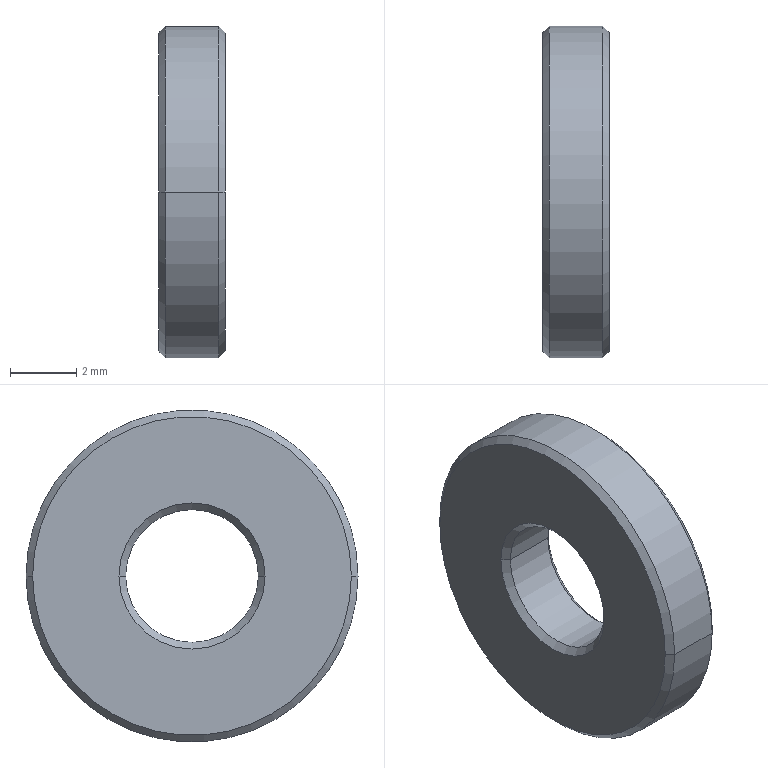Part | STEP file | wasmh10_4_2_2_03 | 1 solid | 14 faces | box 2 x 10 x 10 mm | volume 130.188 mm3 | cone 8 | cylinder 4 | plane 2 | commonest cylinder face diameters 4 x2 10 x2
STEP:
#1=CARTESIAN_POINT('',(0.,0.,0.));
#2=DIRECTION('',(0.,0.,1.));
#3=DIRECTION('',(1.,0.,0.));
#4=AXIS2_PLACEMENT_3D('',#1,#2,#3);
#5=CARTESIAN_POINT('',(2.,4.8,0.));
#6=VERTEX_POINT('',#5);
#7=CARTESIAN_POINT('',(2.,-4.8,0.));
#8=VERTEX_POINT('',#7);
#9=CARTESIAN_POINT('',(2.,0.,0.));
#10=DIRECTION('',(1.,0.,0.));
#11=DIRECTION('',(0.,-1.,0.));
#12=AXIS2_PLACEMENT_3D('',#9,#10,#11);
#13=CIRCLE('',#12,4.8);
#14=CARTESIAN_POINT('',(1.8,0.,0.));
#15=DIRECTION('',(-1.,0.,0.));
#16=DIRECTION('',(0.,-1.,0.));
#17=AXIS2_PLACEMENT_3D('',#14,#15,#16);
#18=CONICAL_SURFACE('',#17,5.,0.7854);
#19=CARTESIAN_POINT('',(6.283,-0.2));
#20=DIRECTION('',(-1.,0.));
#21=VECTOR('',#20,1.);
#22=LINE('',#19,#21);
#23=(GEOMETRIC_REPRESENTATION_CONTEXT(2)PARAMETRIC_REPRESENTATION_CONTEXT()REPRESENTATION_CONTEXT('',''));
#24=DEFINITIONAL_REPRESENTATION('',(#22),#23);
#25=PCURVE('',#18,#24);
#26=CARTESIAN_POINT('',(2.,-3.5,0.));
#27=DIRECTION('',(1.,0.,0.));
#28=DIRECTION('',(0.,1.,0.));
#29=AXIS2_PLACEMENT_3D('',#26,#27,#28);
#30=PLANE('',#29);
#31=CARTESIAN_POINT('',(3.5,0.));
#32=DIRECTION('',(-1.,0.));
#33=AXIS2_PLACEMENT_2D('',#31,#32);
#34=CIRCLE('',#33,4.8);
#35=(GEOMETRIC_REPRESENTATION_CONTEXT(2)PARAMETRIC_REPRESENTATION_CONTEXT()REPRESENTATION_CONTEXT('',''));
#36=DEFINITIONAL_REPRESENTATION('',(#34),#35);
#37=PCURVE('',#30,#36);
#38=SURFACE_CURVE('',#13,(#25,#37),.PCURVE_S1.);
#39=EDGE_CURVE('',#6,#8,#38,.T.);
#40=ORIENTED_EDGE('',*,*,#39,.F.);
#41=CARTESIAN_POINT('',(1.8,5.,0.));
#42=VERTEX_POINT('',#41);
#43=CARTESIAN_POINT('',(1.8,5.,0.));
#44=DIRECTION('',(-0.7071,0.7071,0.));
#45=VECTOR('',#44,1.);
#46=LINE('',#43,#45);
#47=CARTESIAN_POINT('',(3.142,0.));
#48=DIRECTION('',(0.,1.));
#49=VECTOR('',#48,1.);
#50=LINE('',#47,#49);
#51=(GEOMETRIC_REPRESENTATION_CONTEXT(2)PARAMETRIC_REPRESENTATION_CONTEXT()REPRESENTATION_CONTEXT('',''));
#52=DEFINITIONAL_REPRESENTATION('',(#50),#51);
#53=PCURVE('',#18,#52);
#54=CARTESIAN_POINT('',(1.8,0.,0.));
#55=DIRECTION('',(-1.,0.,0.));
#56=DIRECTION('',(0.,-1.,0.));
#57=AXIS2_PLACEMENT_3D('',#54,#55,#56);
#58=CONICAL_SURFACE('',#57,5.,0.7854);
#59=CARTESIAN_POINT('',(3.142,0.));
#60=DIRECTION('',(0.,1.));
#61=VECTOR('',#60,1.);
#62=LINE('',#59,#61);
#63=(GEOMETRIC_REPRESENTATION_CONTEXT(2)PARAMETRIC_REPRESENTATION_CONTEXT()REPRESENTATION_CONTEXT('',''));
#64=DEFINITIONAL_REPRESENTATION('',(#62),#63);
#65=PCURVE('',#58,#64);
#66=SURFACE_CURVE('',#46,(#53,#65),.PCURVE_S1.);
#67=EDGE_CURVE('',#6,#42,#66,.T.);
#68=ORIENTED_EDGE('',*,*,#67,.T.);
#69=CARTESIAN_POINT('',(1.8,-5.,0.));
#70=VERTEX_POINT('',#69);
#71=CARTESIAN_POINT('',(1.8,0.,0.));
#72=DIRECTION('',(1.,0.,0.));
#73=DIRECTION('',(0.,-1.,0.));
#74=AXIS2_PLACEMENT_3D('',#71,#72,#73);
#75=CIRCLE('',#74,5.);
#76=CARTESIAN_POINT('',(6.283,0.));
#77=DIRECTION('',(-1.,0.));
#78=VECTOR('',#77,1.);
#79=LINE('',#76,#78);
#80=(GEOMETRIC_REPRESENTATION_CONTEXT(2)PARAMETRIC_REPRESENTATION_CONTEXT()REPRESENTATION_CONTEXT('',''));
#81=DEFINITIONAL_REPRESENTATION('',(#79),#80);
#82=PCURVE('',#18,#81);
#83=CARTESIAN_POINT('',(1.,0.,0.));
#84=DIRECTION('',(-1.,0.,0.));
#85=DIRECTION('',(0.,-1.,0.));
#86=AXIS2_PLACEMENT_3D('',#83,#84,#85);
#87=CYLINDRICAL_SURFACE('',#86,5.);
#88=CARTESIAN_POINT('',(6.283,-0.8));
#89=DIRECTION('',(-1.,0.));
#90=VECTOR('',#89,1.);
#91=LINE('',#88,#90);
#92=(GEOMETRIC_REPRESENTATION_CONTEXT(2)PARAMETRIC_REPRESENTATION_CONTEXT()REPRESENTATION_CONTEXT('',''));
#93=DEFINITIONAL_REPRESENTATION('',(#91),#92);
#94=PCURVE('',#87,#93);
#95=SURFACE_CURVE('',#75,(#82,#94),.PCURVE_S1.);
#96=EDGE_CURVE('',#42,#70,#95,.T.);
#97=ORIENTED_EDGE('',*,*,#96,.T.);
#98=CARTESIAN_POINT('',(1.8,-5.,0.));
#99=DIRECTION('',(-0.7071,-0.7071,0.));
#100=VECTOR('',#99,1.);
#101=LINE('',#98,#100);
#102=CARTESIAN_POINT('',(0.,0.));
#103=DIRECTION('',(0.,1.));
#104=VECTOR('',#103,1.);
#105=LINE('',#102,#104);
#106=(GEOMETRIC_REPRESENTATION_CONTEXT(2)PARAMETRIC_REPRESENTATION_CONTEXT()REPRESENTATION_CONTEXT('',''));
#107=DEFINITIONAL_REPRESENTATION('',(#105),#106);
#108=PCURVE('',#18,#107);
#109=CARTESIAN_POINT('',(6.283,0.));
#110=DIRECTION('',(0.,1.));
#111=VECTOR('',#110,1.);
#112=LINE('',#109,#111);
#113=(GEOMETRIC_REPRESENTATION_CONTEXT(2)PARAMETRIC_REPRESENTATION_CONTEXT()REPRESENTATION_CONTEXT('',''));
#114=DEFINITIONAL_REPRESENTATION('',(#112),#113);
#115=PCURVE('',#58,#114);
#116=SURFACE_CURVE('',#101,(#108,#115),.PCURVE_S1.);
#117=EDGE_CURVE('',#8,#70,#116,.T.);
#118=ORIENTED_EDGE('',*,*,#117,.F.);
#119=EDGE_LOOP('',(#40,#68,#97,#118));
#120=FACE_BOUND('',#119,.T.);
#121=ADVANCED_FACE('',(#120),#18,.T.);
#122=CARTESIAN_POINT('',(1.8,2.,0.));
#123=VERTEX_POINT('',#122);
#124=CARTESIAN_POINT('',(2.,2.2,0.));
#125=VERTEX_POINT('',#124);
#126=CARTESIAN_POINT('',(2.,2.2,0.));
#127=DIRECTION('',(0.7071,0.7071,0.));
#128=VECTOR('',#127,1.);
#129=LINE('',#126,#128);
#130=CARTESIAN_POINT('',(2.,0.,0.));
#131=DIRECTION('',(1.,0.,0.));
#132=DIRECTION('',(0.,1.,0.));
#133=AXIS2_PLACEMENT_3D('',#130,#131,#132);
#134=CONICAL_SURFACE('',#133,2.2,0.7854);
#135=CARTESIAN_POINT('',(6.283,0.));
#136=DIRECTION('',(0.,1.));
#137=VECTOR('',#136,1.);
#138=LINE('',#135,#137);
#139=(GEOMETRIC_REPRESENTATION_CONTEXT(2)PARAMETRIC_REPRESENTATION_CONTEXT()REPRESENTATION_CONTEXT('',''));
#140=DEFINITIONAL_REPRESENTATION('',(#138),#139);
#141=PCURVE('',#134,#140);
#142=CARTESIAN_POINT('',(2.,0.,0.));
#143=DIRECTION('',(1.,0.,0.));
#144=DIRECTION('',(0.,1.,0.));
#145=AXIS2_PLACEMENT_3D('',#142,#143,#144);
#146=CONICAL_SURFACE('',#145,2.2,0.7854);
#147=CARTESIAN_POINT('',(0.,0.));
#148=DIRECTION('',(0.,1.));
#149=VECTOR('',#148,1.);
#150=LINE('',#147,#149);
#151=(GEOMETRIC_REPRESENTATION_CONTEXT(2)PARAMETRIC_REPRESENTATION_CONTEXT()REPRESENTATION_CONTEXT('',''));
#152=DEFINITIONAL_REPRESENTATION('',(#150),#151);
#153=PCURVE('',#146,#152);
#154=SURFACE_CURVE('',#129,(#141,#153),.PCURVE_S1.);
#155=EDGE_CURVE('',#123,#125,#154,.T.);
#156=ORIENTED_EDGE('',*,*,#155,.T.);
#157=CARTESIAN_POINT('',(2.,-2.2,0.));
#158=VERTEX_POINT('',#157);
#159=CARTESIAN_POINT('',(2.,0.,0.));
#160=DIRECTION('',(-1.,0.,0.));
#161=DIRECTION('',(0.,1.,0.));
#162=AXIS2_PLACEMENT_3D('',#159,#160,#161);
#163=CIRCLE('',#162,2.2);
#164=CARTESIAN_POINT('',(6.283,0.));
#165=DIRECTION('',(-1.,0.));
#166=VECTOR('',#165,1.);
#167=LINE('',#164,#166);
#168=(GEOMETRIC_REPRESENTATION_CONTEXT(2)PARAMETRIC_REPRESENTATION_CONTEXT()REPRESENTATION_CONTEXT('',''));
#169=DEFINITIONAL_REPRESENTATION('',(#167),#168);
#170=PCURVE('',#134,#169);
#171=CARTESIAN_POINT('',(5.7,0.));
#172=CARTESIAN_POINT('',(5.7,-3.811));
#173=CARTESIAN_POINT('',(2.4,-1.905));
#174=CARTESIAN_POINT('',(-0.9,0.));
#175=CARTESIAN_POINT('',(2.4,1.905));
#176=CARTESIAN_POINT('',(5.7,3.811));
#177=CARTESIAN_POINT('',(5.7,0.));
#178=(BOUNDED_CURVE()B_SPLINE_CURVE(2,(#171,#172,#173,#174,#175,#176,#177),.UNSPECIFIED.,.T.,.F.)B_SPLINE_CURVE_WITH_KNOTS((1,2,2,2,2,1),(-2.094,0.,2.094,4.189,6.283,8.378),.UNSPECIFIED.)CURVE()GEOMETRIC_REPRESENTATION_ITEM()RATIONAL_B_SPLINE_CURVE((1.,0.5,1.,0.5,1.,0.5,1.))REPRESENTATION_ITEM(''));
#179=(GEOMETRIC_REPRESENTATION_CONTEXT(2)PARAMETRIC_REPRESENTATION_CONTEXT()REPRESENTATION_CONTEXT('',''));
#180=DEFINITIONAL_REPRESENTATION('',(#178),#179);
#181=PCURVE('',#30,#180);
#182=SURFACE_CURVE('',#163,(#170,#181),.PCURVE_S1.);
#183=EDGE_CURVE('',#125,#158,#182,.T.);
#184=ORIENTED_EDGE('',*,*,#183,.T.);
#185=CARTESIAN_POINT('',(1.8,-2.,0.));
#186=VERTEX_POINT('',#185);
#187=CARTESIAN_POINT('',(2.,-2.2,0.));
#188=DIRECTION('',(0.7071,-0.7071,0.));
#189=VECTOR('',#188,1.);
#190=LINE('',#187,#189);
#191=CARTESIAN_POINT('',(3.142,0.));
#192=DIRECTION('',(0.,1.));
#193=VECTOR('',#192,1.);
#194=LINE('',#191,#193);
#195=(GEOMETRIC_REPRESENTATION_CONTEXT(2)PARAMETRIC_REPRESENTATION_CONTEXT()REPRESENTATION_CONTEXT('',''));
#196=DEFINITIONAL_REPRESENTATION('',(#194),#195);
#197=PCURVE('',#134,#196);
#198=CARTESIAN_POINT('',(3.142,0.));
#199=DIRECTION('',(0.,1.));
#200=VECTOR('',#199,1.);
#201=LINE('',#198,#200);
#202=(GEOMETRIC_REPRESENTATION_CONTEXT(2)PARAMETRIC_REPRESENTATION_CONTEXT()REPRESENTATION_CONTEXT('',''));
#203=DEFINITIONAL_REPRESENTATION('',(#201),#202);
#204=PCURVE('',#146,#203);
#205=SURFACE_CURVE('',#190,(#197,#204),.PCURVE_S1.);
#206=EDGE_CURVE('',#186,#158,#205,.T.);
#207=ORIENTED_EDGE('',*,*,#206,.F.);
#208=CARTESIAN_POINT('',(1.8,0.,0.));
#209=DIRECTION('',(1.,0.,0.));
#210=DIRECTION('',(0.,-1.,0.));
#211=AXIS2_PLACEMENT_3D('',#208,#209,#210);
#212=CIRCLE('',#211,2.);
#213=CARTESIAN_POINT('',(3.142,-0.2));
#214=DIRECTION('',(1.,0.));
#215=VECTOR('',#214,1.);
#216=LINE('',#213,#215);
#217=(GEOMETRIC_REPRESENTATION_CONTEXT(2)PARAMETRIC_REPRESENTATION_CONTEXT()REPRESENTATION_CONTEXT('',''));
#218=DEFINITIONAL_REPRESENTATION('',(#216),#217);
#219=PCURVE('',#134,#218);
#220=CARTESIAN_POINT('',(1.,0.,0.));
#221=DIRECTION('',(-1.,0.,0.));
#222=DIRECTION('',(0.,-1.,0.));
#223=AXIS2_PLACEMENT_3D('',#220,#221,#222);
#224=CYLINDRICAL_SURFACE('',#223,2.);
#225=CARTESIAN_POINT('',(6.283,-0.8));
#226=DIRECTION('',(-1.,0.));
#227=VECTOR('',#226,1.);
#228=LINE('',#225,#227);
#229=(GEOMETRIC_REPRESENTATION_CONTEXT(2)PARAMETRIC_REPRESENTATION_CONTEXT()REPRESENTATION_CONTEXT('',''));
#230=DEFINITIONAL_REPRESENTATION('',(#228),#229);
#231=PCURVE('',#224,#230);
#232=SURFACE_CURVE('',#212,(#219,#231),.PCURVE_S1.);
#233=EDGE_CURVE('',#186,#123,#232,.T.);
#234=ORIENTED_EDGE('',*,*,#233,.T.);
#235=EDGE_LOOP('',(#156,#184,#207,#234));
#236=FACE_BOUND('',#235,.F.);
#237=ADVANCED_FACE('',(#236),#134,.F.);
#238=ORIENTED_EDGE('',*,*,#96,.F.);
#239=CARTESIAN_POINT('',(0.2,5.,0.));
#240=VERTEX_POINT('',#239);
#241=CARTESIAN_POINT('',(1.,5.,0.));
#242=DIRECTION('',(-1.,0.,0.));
#243=VECTOR('',#242,1.);
#244=LINE('',#241,#243);
#245=CARTESIAN_POINT('',(3.142,0.));
#246=DIRECTION('',(0.,1.));
#247=VECTOR('',#246,1.);
#248=LINE('',#245,#247);
#249=(GEOMETRIC_REPRESENTATION_CONTEXT(2)PARAMETRIC_REPRESENTATION_CONTEXT()REPRESENTATION_CONTEXT('',''));
#250=DEFINITIONAL_REPRESENTATION('',(#248),#249);
#251=PCURVE('',#87,#250);
#252=CARTESIAN_POINT('',(1.,0.,0.));
#253=DIRECTION('',(-1.,0.,0.));
#254=DIRECTION('',(0.,-1.,0.));
#255=AXIS2_PLACEMENT_3D('',#252,#253,#254);
#256=CYLINDRICAL_SURFACE('',#255,5.);
#257=CARTESIAN_POINT('',(3.142,0.));
#258=DIRECTION('',(0.,1.));
#259=VECTOR('',#258,1.);
#260=LINE('',#257,#259);
#261=(GEOMETRIC_REPRESENTATION_CONTEXT(2)PARAMETRIC_REPRESENTATION_CONTEXT()REPRESENTATION_CONTEXT('',''));
#262=DEFINITIONAL_REPRESENTATION('',(#260),#261);
#263=PCURVE('',#256,#262);
#264=SURFACE_CURVE('',#244,(#251,#263),.PCURVE_S1.);
#265=EDGE_CURVE('',#42,#240,#264,.T.);
#266=ORIENTED_EDGE('',*,*,#265,.T.);
#267=CARTESIAN_POINT('',(0.2,-5.,0.));
#268=VERTEX_POINT('',#267);
#269=CARTESIAN_POINT('',(0.2,0.,0.));
#270=DIRECTION('',(1.,0.,0.));
#271=DIRECTION('',(0.,-1.,0.));
#272=AXIS2_PLACEMENT_3D('',#269,#270,#271);
#273=CIRCLE('',#272,5.);
#274=CARTESIAN_POINT('',(6.283,0.8));
#275=DIRECTION('',(-1.,0.));
#276=VECTOR('',#275,1.);
#277=LINE('',#274,#276);
#278=(GEOMETRIC_REPRESENTATION_CONTEXT(2)PARAMETRIC_REPRESENTATION_CONTEXT()REPRESENTATION_CONTEXT('',''));
#279=DEFINITIONAL_REPRESENTATION('',(#277),#278);
#280=PCURVE('',#87,#279);
#281=CARTESIAN_POINT('',(0.2,0.,0.));
#282=DIRECTION('',(1.,0.,0.));
#283=DIRECTION('',(0.,1.,0.));
#284=AXIS2_PLACEMENT_3D('',#281,#282,#283);
#285=CONICAL_SURFACE('',#284,5.,0.7854);
#286=CARTESIAN_POINT('',(-3.142,0.));
#287=DIRECTION('',(1.,0.));
#288=VECTOR('',#287,1.);
#289=LINE('',#286,#288);
#290=(GEOMETRIC_REPRESENTATION_CONTEXT(2)PARAMETRIC_REPRESENTATION_CONTEXT()REPRESENTATION_CONTEXT('',''));
#291=DEFINITIONAL_REPRESENTATION('',(#289),#290);
#292=PCURVE('',#285,#291);
#293=SURFACE_CURVE('',#273,(#280,#292),.PCURVE_S1.);
#294=EDGE_CURVE('',#240,#268,#293,.T.);
#295=ORIENTED_EDGE('',*,*,#294,.T.);
#296=CARTESIAN_POINT('',(1.,-5.,0.));
#297=DIRECTION('',(-1.,0.,0.));
#298=VECTOR('',#297,1.);
#299=LINE('',#296,#298);
#300=CARTESIAN_POINT('',(0.,0.));
#301=DIRECTION('',(0.,1.));
#302=VECTOR('',#301,1.);
#303=LINE('',#300,#302);
#304=(GEOMETRIC_REPRESENTATION_CONTEXT(2)PARAMETRIC_REPRESENTATION_CONTEXT()REPRESENTATION_CONTEXT('',''));
#305=DEFINITIONAL_REPRESENTATION('',(#303),#304);
#306=PCURVE('',#87,#305);
#307=CARTESIAN_POINT('',(6.283,0.));
#308=DIRECTION('',(0.,1.));
#309=VECTOR('',#308,1.);
#310=LINE('',#307,#309);
#311=(GEOMETRIC_REPRESENTATION_CONTEXT(2)PARAMETRIC_REPRESENTATION_CONTEXT()REPRESENTATION_CONTEXT('',''));
#312=DEFINITIONAL_REPRESENTATION('',(#310),#311);
#313=PCURVE('',#256,#312);
#314=SURFACE_CURVE('',#299,(#306,#313),.PCURVE_S1.);
#315=EDGE_CURVE('',#70,#268,#314,.T.);
#316=ORIENTED_EDGE('',*,*,#315,.F.);
#317=EDGE_LOOP('',(#238,#266,#295,#316));
#318=FACE_BOUND('',#317,.T.);
#319=ADVANCED_FACE('',(#318),#87,.T.);
#320=CARTESIAN_POINT('',(0.2,-2.,0.));
#321=VERTEX_POINT('',#320);
#322=CARTESIAN_POINT('',(1.,-2.,0.));
#323=DIRECTION('',(-1.,0.,0.));
#324=VECTOR('',#323,1.);
#325=LINE('',#322,#324);
#326=CARTESIAN_POINT('',(6.283,0.));
#327=DIRECTION('',(0.,1.));
#328=VECTOR('',#327,1.);
#329=LINE('',#326,#328);
#330=(GEOMETRIC_REPRESENTATION_CONTEXT(2)PARAMETRIC_REPRESENTATION_CONTEXT()REPRESENTATION_CONTEXT('',''));
#331=DEFINITIONAL_REPRESENTATION('',(#329),#330);
#332=PCURVE('',#224,#331);
#333=CARTESIAN_POINT('',(1.,0.,0.));
#334=DIRECTION('',(-1.,0.,0.));
#335=DIRECTION('',(0.,-1.,0.));
#336=AXIS2_PLACEMENT_3D('',#333,#334,#335);
#337=CYLINDRICAL_SURFACE('',#336,2.);
#338=CARTESIAN_POINT('',(0.,0.));
#339=DIRECTION('',(0.,1.));
#340=VECTOR('',#339,1.);
#341=LINE('',#338,#340);
#342=(GEOMETRIC_REPRESENTATION_CONTEXT(2)PARAMETRIC_REPRESENTATION_CONTEXT()REPRESENTATION_CONTEXT('',''));
#343=DEFINITIONAL_REPRESENTATION('',(#341),#342);
#344=PCURVE('',#337,#343);
#345=SURFACE_CURVE('',#325,(#332,#344),.PCURVE_S1.);
#346=EDGE_CURVE('',#186,#321,#345,.T.);
#347=ORIENTED_EDGE('',*,*,#346,.T.);
#348=CARTESIAN_POINT('',(0.2,2.,0.));
#349=VERTEX_POINT('',#348);
#350=CARTESIAN_POINT('',(0.2,0.,0.));
#351=DIRECTION('',(1.,0.,0.));
#352=DIRECTION('',(0.,-1.,0.));
#353=AXIS2_PLACEMENT_3D('',#350,#351,#352);
#354=CIRCLE('',#353,2.);
#355=CARTESIAN_POINT('',(6.283,0.8));
#356=DIRECTION('',(-1.,0.));
#357=VECTOR('',#356,1.);
#358=LINE('',#355,#357);
#359=(GEOMETRIC_REPRESENTATION_CONTEXT(2)PARAMETRIC_REPRESENTATION_CONTEXT()REPRESENTATION_CONTEXT('',''));
#360=DEFINITIONAL_REPRESENTATION('',(#358),#359);
#361=PCURVE('',#224,#360);
#362=CARTESIAN_POINT('',(0.,0.,0.));
#363=DIRECTION('',(-1.,0.,0.));
#364=DIRECTION('',(0.,-1.,0.));
#365=AXIS2_PLACEMENT_3D('',#362,#363,#364);
#366=CONICAL_SURFACE('',#365,2.2,0.7854);
#367=CARTESIAN_POINT('',(6.283,-0.2));
#368=DIRECTION('',(-1.,0.));
#369=VECTOR('',#368,1.);
#370=LINE('',#367,#369);
#371=(GEOMETRIC_REPRESENTATION_CONTEXT(2)PARAMETRIC_REPRESENTATION_CONTEXT()REPRESENTATION_CONTEXT('',''));
#372=DEFINITIONAL_REPRESENTATION('',(#370),#371);
#373=PCURVE('',#366,#372);
#374=SURFACE_CURVE('',#354,(#361,#373),.PCURVE_S1.);
#375=EDGE_CURVE('',#321,#349,#374,.T.);
#376=ORIENTED_EDGE('',*,*,#375,.T.);
#377=CARTESIAN_POINT('',(1.,2.,0.));
#378=DIRECTION('',(-1.,0.,0.));
#379=VECTOR('',#378,1.);
#380=LINE('',#377,#379);
#381=CARTESIAN_POINT('',(3.142,0.));
#382=DIRECTION('',(0.,1.));
#383=VECTOR('',#382,1.);
#384=LINE('',#381,#383);
#385=(GEOMETRIC_REPRESENTATION_CONTEXT(2)PARAMETRIC_REPRESENTATION_CONTEXT()REPRESENTATION_CONTEXT('',''));
#386=DEFINITIONAL_REPRESENTATION('',(#384),#385);
#387=PCURVE('',#224,#386);
#388=CARTESIAN_POINT('',(3.142,0.));
#389=DIRECTION('',(0.,1.));
#390=VECTOR('',#389,1.);
#391=LINE('',#388,#390);
#392=(GEOMETRIC_REPRESENTATION_CONTEXT(2)PARAMETRIC_REPRESENTATION_CONTEXT()REPRESENTATION_CONTEXT('',''));
#393=DEFINITIONAL_REPRESENTATION('',(#391),#392);
#394=PCURVE('',#337,#393);
#395=SURFACE_CURVE('',#380,(#387,#394),.PCURVE_S1.);
#396=EDGE_CURVE('',#123,#349,#395,.T.);
#397=ORIENTED_EDGE('',*,*,#396,.F.);
#398=ORIENTED_EDGE('',*,*,#233,.F.);
#399=EDGE_LOOP('',(#347,#376,#397,#398));
#400=FACE_BOUND('',#399,.F.);
#401=ADVANCED_FACE('',(#400),#224,.F.);
#402=CARTESIAN_POINT('',(0.,4.8,0.));
#403=VERTEX_POINT('',#402);
#404=CARTESIAN_POINT('',(0.,-4.8,0.));
#405=VERTEX_POINT('',#404);
#406=CARTESIAN_POINT('',(0.,0.,0.));
#407=DIRECTION('',(1.,0.,0.));
#408=DIRECTION('',(0.,1.,0.));
#409=AXIS2_PLACEMENT_3D('',#406,#407,#408);
#410=CIRCLE('',#409,4.8);
#411=CARTESIAN_POINT('',(0.,-0.2));
#412=DIRECTION('',(1.,0.));
#413=VECTOR('',#412,1.);
#414=LINE('',#411,#413);
#415=(GEOMETRIC_REPRESENTATION_CONTEXT(2)PARAMETRIC_REPRESENTATION_CONTEXT()REPRESENTATION_CONTEXT('',''));
#416=DEFINITIONAL_REPRESENTATION('',(#414),#415);
#417=PCURVE('',#285,#416);
#418=CARTESIAN_POINT('',(0.,-3.5,0.));
#419=DIRECTION('',(-1.,0.,0.));
#420=DIRECTION('',(0.,-1.,0.));
#421=AXIS2_PLACEMENT_3D('',#418,#419,#420);
#422=PLANE('',#421);
#423=CARTESIAN_POINT('',(-8.3,0.));
#424=CARTESIAN_POINT('',(-8.3,8.314));
#425=CARTESIAN_POINT('',(-1.1,4.157));
#426=CARTESIAN_POINT('',(6.1,0.));
#427=CARTESIAN_POINT('',(-1.1,-4.157));
#428=CARTESIAN_POINT('',(-8.3,-8.314));
#429=CARTESIAN_POINT('',(-8.3,0.));
#430=(BOUNDED_CURVE()B_SPLINE_CURVE(2,(#423,#424,#425,#426,#427,#428,#429),.UNSPECIFIED.,.T.,.F.)B_SPLINE_CURVE_WITH_KNOTS((1,2,2,2,2,1),(-2.094,0.,2.094,4.189,6.283,8.378),.UNSPECIFIED.)CURVE()GEOMETRIC_REPRESENTATION_ITEM()RATIONAL_B_SPLINE_CURVE((1.,0.5,1.,0.5,1.,0.5,1.))REPRESENTATION_ITEM(''));
#431=(GEOMETRIC_REPRESENTATION_CONTEXT(2)PARAMETRIC_REPRESENTATION_CONTEXT()REPRESENTATION_CONTEXT('',''));
#432=DEFINITIONAL_REPRESENTATION('',(#430),#431);
#433=PCURVE('',#422,#432);
#434=SURFACE_CURVE('',#410,(#417,#433),.PCURVE_S1.);
#435=EDGE_CURVE('',#403,#405,#434,.T.);
#436=ORIENTED_EDGE('',*,*,#435,.T.);
#437=CARTESIAN_POINT('',(0.2,-5.,0.));
#438=DIRECTION('',(0.7071,-0.7071,0.));
#439=VECTOR('',#438,1.);
#440=LINE('',#437,#439);
#441=CARTESIAN_POINT('',(3.142,0.));
#442=DIRECTION('',(0.,1.));
#443=VECTOR('',#442,1.);
#444=LINE('',#441,#443);
#445=(GEOMETRIC_REPRESENTATION_CONTEXT(2)PARAMETRIC_REPRESENTATION_CONTEXT()REPRESENTATION_CONTEXT('',''));
#446=DEFINITIONAL_REPRESENTATION('',(#444),#445);
#447=PCURVE('',#285,#446);
#448=CARTESIAN_POINT('',(0.2,0.,0.));
#449=DIRECTION('',(1.,0.,0.));
#450=DIRECTION('',(0.,1.,0.));
#451=AXIS2_PLACEMENT_3D('',#448,#449,#450);
#452=CONICAL_SURFACE('',#451,5.,0.7854);
#453=CARTESIAN_POINT('',(3.142,0.));
#454=DIRECTION('',(0.,1.));
#455=VECTOR('',#454,1.);
#456=LINE('',#453,#455);
#457=(GEOMETRIC_REPRESENTATION_CONTEXT(2)PARAMETRIC_REPRESENTATION_CONTEXT()REPRESENTATION_CONTEXT('',''));
#458=DEFINITIONAL_REPRESENTATION('',(#456),#457);
#459=PCURVE('',#452,#458);
#460=SURFACE_CURVE('',#440,(#447,#459),.PCURVE_S1.);
#461=EDGE_CURVE('',#405,#268,#460,.T.);
#462=ORIENTED_EDGE('',*,*,#461,.T.);
#463=ORIENTED_EDGE('',*,*,#294,.F.);
#464=CARTESIAN_POINT('',(0.2,5.,0.));
#465=DIRECTION('',(0.7071,0.7071,0.));
#466=VECTOR('',#465,1.);
#467=LINE('',#464,#466);
#468=CARTESIAN_POINT('',(0.,0.));
#469=DIRECTION('',(0.,1.));
#470=VECTOR('',#469,1.);
#471=LINE('',#468,#470);
#472=(GEOMETRIC_REPRESENTATION_CONTEXT(2)PARAMETRIC_REPRESENTATION_CONTEXT()REPRESENTATION_CONTEXT('',''));
#473=DEFINITIONAL_REPRESENTATION('',(#471),#472);
#474=PCURVE('',#285,#473);
#475=CARTESIAN_POINT('',(6.283,0.));
#476=DIRECTION('',(0.,1.));
#477=VECTOR('',#476,1.);
#478=LINE('',#475,#477);
#479=(GEOMETRIC_REPRESENTATION_CONTEXT(2)PARAMETRIC_REPRESENTATION_CONTEXT()REPRESENTATION_CONTEXT('',''));
#480=DEFINITIONAL_REPRESENTATION('',(#478),#479);
#481=PCURVE('',#452,#480);
#482=SURFACE_CURVE('',#467,(#474,#481),.PCURVE_S1.);
#483=EDGE_CURVE('',#403,#240,#482,.T.);
#484=ORIENTED_EDGE('',*,*,#483,.F.);
#485=EDGE_LOOP('',(#436,#462,#463,#484));
#486=FACE_BOUND('',#485,.T.);
#487=ADVANCED_FACE('',(#486),#285,.T.);
#488=CARTESIAN_POINT('',(0.,-2.2,0.));
#489=VERTEX_POINT('',#488);
#490=CARTESIAN_POINT('',(0.,-2.2,0.));
#491=DIRECTION('',(-0.7071,-0.7071,0.));
#492=VECTOR('',#491,1.);
#493=LINE('',#490,#492);
#494=CARTESIAN_POINT('',(6.283,0.));
#495=DIRECTION('',(0.,1.));
#496=VECTOR('',#495,1.);
#497=LINE('',#494,#496);
#498=(GEOMETRIC_REPRESENTATION_CONTEXT(2)PARAMETRIC_REPRESENTATION_CONTEXT()REPRESENTATION_CONTEXT('',''));
#499=DEFINITIONAL_REPRESENTATION('',(#497),#498);
#500=PCURVE('',#366,#499);
#501=CARTESIAN_POINT('',(0.,0.,0.));
#502=DIRECTION('',(-1.,0.,0.));
#503=DIRECTION('',(0.,-1.,0.));
#504=AXIS2_PLACEMENT_3D('',#501,#502,#503);
#505=CONICAL_SURFACE('',#504,2.2,0.7854);
#506=CARTESIAN_POINT('',(0.,0.));
#507=DIRECTION('',(0.,1.));
#508=VECTOR('',#507,1.);
#509=LINE('',#506,#508);
#510=(GEOMETRIC_REPRESENTATION_CONTEXT(2)PARAMETRIC_REPRESENTATION_CONTEXT()REPRESENTATION_CONTEXT('',''));
#511=DEFINITIONAL_REPRESENTATION('',(#509),#510);
#512=PCURVE('',#505,#511);
#513=SURFACE_CURVE('',#493,(#500,#512),.PCURVE_S1.);
#514=EDGE_CURVE('',#321,#489,#513,.T.);
#515=ORIENTED_EDGE('',*,*,#514,.T.);
#516=CARTESIAN_POINT('',(0.,2.2,0.));
#517=VERTEX_POINT('',#516);
#518=CARTESIAN_POINT('',(0.,0.,0.));
#519=DIRECTION('',(1.,0.,0.));
#520=DIRECTION('',(0.,-1.,0.));
#521=AXIS2_PLACEMENT_3D('',#518,#519,#520);
#522=CIRCLE('',#521,2.2);
#523=CARTESIAN_POINT('',(6.283,0.));
#524=DIRECTION('',(-1.,0.));
#525=VECTOR('',#524,1.);
#526=LINE('',#523,#525);
#527=(GEOMETRIC_REPRESENTATION_CONTEXT(2)PARAMETRIC_REPRESENTATION_CONTEXT()REPRESENTATION_CONTEXT('',''));
#528=DEFINITIONAL_REPRESENTATION('',(#526),#527);
#529=PCURVE('',#366,#528);
#530=CARTESIAN_POINT('',(-1.3,0.));
#531=CARTESIAN_POINT('',(-1.3,-3.811));
#532=CARTESIAN_POINT('',(-4.6,-1.905));
#533=CARTESIAN_POINT('',(-7.9,0.));
#534=CARTESIAN_POINT('',(-4.6,1.905));
#535=CARTESIAN_POINT('',(-1.3,3.811));
#536=CARTESIAN_POINT('',(-1.3,0.));
#537=(BOUNDED_CURVE()B_SPLINE_CURVE(2,(#530,#531,#532,#533,#534,#535,#536),.UNSPECIFIED.,.T.,.F.)B_SPLINE_CURVE_WITH_KNOTS((1,2,2,2,2,1),(-2.094,0.,2.094,4.189,6.283,8.378),.UNSPECIFIED.)CURVE()GEOMETRIC_REPRESENTATION_ITEM()RATIONAL_B_SPLINE_CURVE((1.,0.5,1.,0.5,1.,0.5,1.))REPRESENTATION_ITEM(''));
#538=(GEOMETRIC_REPRESENTATION_CONTEXT(2)PARAMETRIC_REPRESENTATION_CONTEXT()REPRESENTATION_CONTEXT('',''));
#539=DEFINITIONAL_REPRESENTATION('',(#537),#538);
#540=PCURVE('',#422,#539);
#541=SURFACE_CURVE('',#522,(#529,#540),.PCURVE_S1.);
#542=EDGE_CURVE('',#489,#517,#541,.T.);
#543=ORIENTED_EDGE('',*,*,#542,.T.);
#544=CARTESIAN_POINT('',(0.,2.2,0.));
#545=DIRECTION('',(-0.7071,0.7071,0.));
#546=VECTOR('',#545,1.);
#547=LINE('',#544,#546);
#548=CARTESIAN_POINT('',(3.142,0.));
#549=DIRECTION('',(0.,1.));
#550=VECTOR('',#549,1.);
#551=LINE('',#548,#550);
#552=(GEOMETRIC_REPRESENTATION_CONTEXT(2)PARAMETRIC_REPRESENTATION_CONTEXT()REPRESENTATION_CONTEXT('',''));
#553=DEFINITIONAL_REPRESENTATION('',(#551),#552);
#554=PCURVE('',#366,#553);
#555=CARTESIAN_POINT('',(3.142,0.));
#556=DIRECTION('',(0.,1.));
#557=VECTOR('',#556,1.);
#558=LINE('',#555,#557);
#559=(GEOMETRIC_REPRESENTATION_CONTEXT(2)PARAMETRIC_REPRESENTATION_CONTEXT()REPRESENTATION_CONTEXT('',''));
#560=DEFINITIONAL_REPRESENTATION('',(#558),#559);
#561=PCURVE('',#505,#560);
#562=SURFACE_CURVE('',#547,(#554,#561),.PCURVE_S1.);
#563=EDGE_CURVE('',#349,#517,#562,.T.);
#564=ORIENTED_EDGE('',*,*,#563,.F.);
#565=ORIENTED_EDGE('',*,*,#375,.F.);
#566=EDGE_LOOP('',(#515,#543,#564,#565));
#567=FACE_BOUND('',#566,.F.);
#568=ADVANCED_FACE('',(#567),#366,.F.);
#569=CARTESIAN_POINT('',(2.,0.,0.));
#570=DIRECTION('',(1.,0.,0.));
#571=DIRECTION('',(0.,-1.,0.));
#572=AXIS2_PLACEMENT_3D('',#569,#570,#571);
#573=CIRCLE('',#572,4.8);
#574=CARTESIAN_POINT('',(3.5,0.));
#575=DIRECTION('',(-1.,0.));
#576=AXIS2_PLACEMENT_2D('',#574,#575);
#577=CIRCLE('',#576,4.8);
#578=(GEOMETRIC_REPRESENTATION_CONTEXT(2)PARAMETRIC_REPRESENTATION_CONTEXT()REPRESENTATION_CONTEXT('',''));
#579=DEFINITIONAL_REPRESENTATION('',(#577),#578);
#580=PCURVE('',#30,#579);
#581=CARTESIAN_POINT('',(6.283,-0.2));
#582=DIRECTION('',(-1.,0.));
#583=VECTOR('',#582,1.);
#584=LINE('',#581,#583);
#585=(GEOMETRIC_REPRESENTATION_CONTEXT(2)PARAMETRIC_REPRESENTATION_CONTEXT()REPRESENTATION_CONTEXT('',''));
#586=DEFINITIONAL_REPRESENTATION('',(#584),#585);
#587=PCURVE('',#58,#586);
#588=SURFACE_CURVE('',#573,(#580,#587),.PCURVE_S1.);
#589=EDGE_CURVE('',#8,#6,#588,.T.);
#590=ORIENTED_EDGE('',*,*,#589,.T.);
#591=ORIENTED_EDGE('',*,*,#39,.T.);
#592=EDGE_LOOP('',(#590,#591));
#593=FACE_BOUND('',#592,.T.);
#594=ORIENTED_EDGE('',*,*,#183,.T.);
#595=CARTESIAN_POINT('',(2.,0.,0.));
#596=DIRECTION('',(-1.,0.,0.));
#597=DIRECTION('',(0.,1.,0.));
#598=AXIS2_PLACEMENT_3D('',#595,#596,#597);
#599=CIRCLE('',#598,2.2);
#600=CARTESIAN_POINT('',(5.7,0.));
#601=CARTESIAN_POINT('',(5.7,-3.811));
#602=CARTESIAN_POINT('',(2.4,-1.905));
#603=CARTESIAN_POINT('',(-0.9,0.));
#604=CARTESIAN_POINT('',(2.4,1.905));
#605=CARTESIAN_POINT('',(5.7,3.811));
#606=CARTESIAN_POINT('',(5.7,0.));
#607=(BOUNDED_CURVE()B_SPLINE_CURVE(2,(#600,#601,#602,#603,#604,#605,#606),.UNSPECIFIED.,.T.,.F.)B_SPLINE_CURVE_WITH_KNOTS((1,2,2,2,2,1),(-2.094,0.,2.094,4.189,6.283,8.378),.UNSPECIFIED.)CURVE()GEOMETRIC_REPRESENTATION_ITEM()RATIONAL_B_SPLINE_CURVE((1.,0.5,1.,0.5,1.,0.5,1.))REPRESENTATION_ITEM(''));
#608=(GEOMETRIC_REPRESENTATION_CONTEXT(2)PARAMETRIC_REPRESENTATION_CONTEXT()REPRESENTATION_CONTEXT('',''));
#609=DEFINITIONAL_REPRESENTATION('',(#607),#608);
#610=PCURVE('',#30,#609);
#611=CARTESIAN_POINT('',(6.283,0.));
#612=DIRECTION('',(-1.,0.));
#613=VECTOR('',#612,1.);
#614=LINE('',#611,#613);
#615=(GEOMETRIC_REPRESENTATION_CONTEXT(2)PARAMETRIC_REPRESENTATION_CONTEXT()REPRESENTATION_CONTEXT('',''));
#616=DEFINITIONAL_REPRESENTATION('',(#614),#615);
#617=PCURVE('',#146,#616);
#618=SURFACE_CURVE('',#599,(#610,#617),.PCURVE_S1.);
#619=EDGE_CURVE('',#158,#125,#618,.T.);
#620=ORIENTED_EDGE('',*,*,#619,.T.);
#621=EDGE_LOOP('',(#594,#620));
#622=FACE_BOUND('',#621,.T.);
#623=ADVANCED_FACE('',(#593,#622),#30,.T.);
#624=ORIENTED_EDGE('',*,*,#67,.F.);
#625=ORIENTED_EDGE('',*,*,#589,.F.);
#626=ORIENTED_EDGE('',*,*,#117,.T.);
#627=CARTESIAN_POINT('',(1.8,0.,0.));
#628=DIRECTION('',(1.,0.,0.));
#629=DIRECTION('',(0.,-1.,0.));
#630=AXIS2_PLACEMENT_3D('',#627,#628,#629);
#631=CIRCLE('',#630,5.);
#632=CARTESIAN_POINT('',(6.283,0.));
#633=DIRECTION('',(-1.,0.));
#634=VECTOR('',#633,1.);
#635=LINE('',#632,#634);
#636=(GEOMETRIC_REPRESENTATION_CONTEXT(2)PARAMETRIC_REPRESENTATION_CONTEXT()REPRESENTATION_CONTEXT('',''));
#637=DEFINITIONAL_REPRESENTATION('',(#635),#636);
#638=PCURVE('',#58,#637);
#639=CARTESIAN_POINT('',(6.283,-0.8));
#640=DIRECTION('',(-1.,0.));
#641=VECTOR('',#640,1.);
#642=LINE('',#639,#641);
#643=(GEOMETRIC_REPRESENTATION_CONTEXT(2)PARAMETRIC_REPRESENTATION_CONTEXT()REPRESENTATION_CONTEXT('',''));
#644=DEFINITIONAL_REPRESENTATION('',(#642),#643);
#645=PCURVE('',#256,#644);
#646=SURFACE_CURVE('',#631,(#638,#645),.PCURVE_S1.);
#647=EDGE_CURVE('',#70,#42,#646,.T.);
#648=ORIENTED_EDGE('',*,*,#647,.T.);
#649=EDGE_LOOP('',(#624,#625,#626,#648));
#650=FACE_BOUND('',#649,.T.);
#651=ADVANCED_FACE('',(#650),#58,.T.);
#652=ORIENTED_EDGE('',*,*,#619,.T.);
#653=ORIENTED_EDGE('',*,*,#155,.F.);
#654=CARTESIAN_POINT('',(1.8,0.,0.));
#655=DIRECTION('',(1.,0.,0.));
#656=DIRECTION('',(0.,-1.,0.));
#657=AXIS2_PLACEMENT_3D('',#654,#655,#656);
#658=CIRCLE('',#657,2.);
#659=CARTESIAN_POINT('',(-3.142,-0.2));
#660=DIRECTION('',(1.,0.));
#661=VECTOR('',#660,1.);
#662=LINE('',#659,#661);
#663=(GEOMETRIC_REPRESENTATION_CONTEXT(2)PARAMETRIC_REPRESENTATION_CONTEXT()REPRESENTATION_CONTEXT('',''));
#664=DEFINITIONAL_REPRESENTATION('',(#662),#663);
#665=PCURVE('',#146,#664);
#666=CARTESIAN_POINT('',(6.283,-0.8));
#667=DIRECTION('',(-1.,0.));
#668=VECTOR('',#667,1.);
#669=LINE('',#666,#668);
#670=(GEOMETRIC_REPRESENTATION_CONTEXT(2)PARAMETRIC_REPRESENTATION_CONTEXT()REPRESENTATION_CONTEXT('',''));
#671=DEFINITIONAL_REPRESENTATION('',(#669),#670);
#672=PCURVE('',#337,#671);
#673=SURFACE_CURVE('',#658,(#665,#672),.PCURVE_S1.);
#674=EDGE_CURVE('',#123,#186,#673,.T.);
#675=ORIENTED_EDGE('',*,*,#674,.T.);
#676=ORIENTED_EDGE('',*,*,#206,.T.);
#677=EDGE_LOOP('',(#652,#653,#675,#676));
#678=FACE_BOUND('',#677,.F.);
#679=ADVANCED_FACE('',(#678),#146,.F.);
#680=ORIENTED_EDGE('',*,*,#265,.F.);
#681=ORIENTED_EDGE('',*,*,#647,.F.);
#682=ORIENTED_EDGE('',*,*,#315,.T.);
#683=CARTESIAN_POINT('',(0.2,0.,0.));
#684=DIRECTION('',(1.,0.,0.));
#685=DIRECTION('',(0.,-1.,0.));
#686=AXIS2_PLACEMENT_3D('',#683,#684,#685);
#687=CIRCLE('',#686,5.);
#688=CARTESIAN_POINT('',(6.283,0.8));
#689=DIRECTION('',(-1.,0.));
#690=VECTOR('',#689,1.);
#691=LINE('',#688,#690);
#692=(GEOMETRIC_REPRESENTATION_CONTEXT(2)PARAMETRIC_REPRESENTATION_CONTEXT()REPRESENTATION_CONTEXT('',''));
#693=DEFINITIONAL_REPRESENTATION('',(#691),#692);
#694=PCURVE('',#256,#693);
#695=CARTESIAN_POINT('',(3.142,0.));
#696=DIRECTION('',(1.,0.));
#697=VECTOR('',#696,1.);
#698=LINE('',#695,#697);
#699=(GEOMETRIC_REPRESENTATION_CONTEXT(2)PARAMETRIC_REPRESENTATION_CONTEXT()REPRESENTATION_CONTEXT('',''));
#700=DEFINITIONAL_REPRESENTATION('',(#698),#699);
#701=PCURVE('',#452,#700);
#702=SURFACE_CURVE('',#687,(#694,#701),.PCURVE_S1.);
#703=EDGE_CURVE('',#268,#240,#702,.T.);
#704=ORIENTED_EDGE('',*,*,#703,.T.);
#705=EDGE_LOOP('',(#680,#681,#682,#704));
#706=FACE_BOUND('',#705,.T.);
#707=ADVANCED_FACE('',(#706),#256,.T.);
#708=CARTESIAN_POINT('',(0.2,0.,0.));
#709=DIRECTION('',(1.,0.,0.));
#710=DIRECTION('',(0.,-1.,0.));
#711=AXIS2_PLACEMENT_3D('',#708,#709,#710);
#712=CIRCLE('',#711,2.);
#713=CARTESIAN_POINT('',(6.283,0.8));
#714=DIRECTION('',(-1.,0.));
#715=VECTOR('',#714,1.);
#716=LINE('',#713,#715);
#717=(GEOMETRIC_REPRESENTATION_CONTEXT(2)PARAMETRIC_REPRESENTATION_CONTEXT()REPRESENTATION_CONTEXT('',''));
#718=DEFINITIONAL_REPRESENTATION('',(#716),#717);
#719=PCURVE('',#337,#718);
#720=CARTESIAN_POINT('',(6.283,-0.2));
#721=DIRECTION('',(-1.,0.));
#722=VECTOR('',#721,1.);
#723=LINE('',#720,#722);
#724=(GEOMETRIC_REPRESENTATION_CONTEXT(2)PARAMETRIC_REPRESENTATION_CONTEXT()REPRESENTATION_CONTEXT('',''));
#725=DEFINITIONAL_REPRESENTATION('',(#723),#724);
#726=PCURVE('',#505,#725);
#727=SURFACE_CURVE('',#712,(#719,#726),.PCURVE_S1.);
#728=EDGE_CURVE('',#349,#321,#727,.T.);
#729=ORIENTED_EDGE('',*,*,#728,.T.);
#730=ORIENTED_EDGE('',*,*,#346,.F.);
#731=ORIENTED_EDGE('',*,*,#674,.F.);
#732=ORIENTED_EDGE('',*,*,#396,.T.);
#733=EDGE_LOOP('',(#729,#730,#731,#732));
#734=FACE_BOUND('',#733,.F.);
#735=ADVANCED_FACE('',(#734),#337,.F.);
#736=ORIENTED_EDGE('',*,*,#461,.F.);
#737=CARTESIAN_POINT('',(0.,0.,0.));
#738=DIRECTION('',(1.,0.,0.));
#739=DIRECTION('',(0.,1.,0.));
#740=AXIS2_PLACEMENT_3D('',#737,#738,#739);
#741=CIRCLE('',#740,4.8);
#742=CARTESIAN_POINT('',(0.,-0.2));
#743=DIRECTION('',(1.,0.));
#744=VECTOR('',#743,1.);
#745=LINE('',#742,#744);
#746=(GEOMETRIC_REPRESENTATION_CONTEXT(2)PARAMETRIC_REPRESENTATION_CONTEXT()REPRESENTATION_CONTEXT('',''));
#747=DEFINITIONAL_REPRESENTATION('',(#745),#746);
#748=PCURVE('',#452,#747);
#749=CARTESIAN_POINT('',(-8.3,0.));
#750=CARTESIAN_POINT('',(-8.3,8.314));
#751=CARTESIAN_POINT('',(-1.1,4.157));
#752=CARTESIAN_POINT('',(6.1,0.));
#753=CARTESIAN_POINT('',(-1.1,-4.157));
#754=CARTESIAN_POINT('',(-8.3,-8.314));
#755=CARTESIAN_POINT('',(-8.3,0.));
#756=(BOUNDED_CURVE()B_SPLINE_CURVE(2,(#749,#750,#751,#752,#753,#754,#755),.UNSPECIFIED.,.T.,.F.)B_SPLINE_CURVE_WITH_KNOTS((1,2,2,2,2,1),(-2.094,0.,2.094,4.189,6.283,8.378),.UNSPECIFIED.)CURVE()GEOMETRIC_REPRESENTATION_ITEM()RATIONAL_B_SPLINE_CURVE((1.,0.5,1.,0.5,1.,0.5,1.))REPRESENTATION_ITEM(''));
#757=(GEOMETRIC_REPRESENTATION_CONTEXT(2)PARAMETRIC_REPRESENTATION_CONTEXT()REPRESENTATION_CONTEXT('',''));
#758=DEFINITIONAL_REPRESENTATION('',(#756),#757);
#759=PCURVE('',#422,#758);
#760=SURFACE_CURVE('',#741,(#748,#759),.PCURVE_S1.);
#761=EDGE_CURVE('',#405,#403,#760,.T.);
#762=ORIENTED_EDGE('',*,*,#761,.T.);
#763=ORIENTED_EDGE('',*,*,#483,.T.);
#764=ORIENTED_EDGE('',*,*,#703,.F.);
#765=EDGE_LOOP('',(#736,#762,#763,#764));
#766=FACE_BOUND('',#765,.T.);
#767=ADVANCED_FACE('',(#766),#452,.T.);
#768=CARTESIAN_POINT('',(0.,0.,0.));
#769=DIRECTION('',(1.,0.,0.));
#770=DIRECTION('',(0.,-1.,0.));
#771=AXIS2_PLACEMENT_3D('',#768,#769,#770);
#772=CIRCLE('',#771,2.2);
#773=CARTESIAN_POINT('',(6.283,0.));
#774=DIRECTION('',(-1.,0.));
#775=VECTOR('',#774,1.);
#776=LINE('',#773,#775);
#777=(GEOMETRIC_REPRESENTATION_CONTEXT(2)PARAMETRIC_REPRESENTATION_CONTEXT()REPRESENTATION_CONTEXT('',''));
#778=DEFINITIONAL_REPRESENTATION('',(#776),#777);
#779=PCURVE('',#505,#778);
#780=CARTESIAN_POINT('',(-1.3,0.));
#781=CARTESIAN_POINT('',(-1.3,-3.811));
#782=CARTESIAN_POINT('',(-4.6,-1.905));
#783=CARTESIAN_POINT('',(-7.9,0.));
#784=CARTESIAN_POINT('',(-4.6,1.905));
#785=CARTESIAN_POINT('',(-1.3,3.811));
#786=CARTESIAN_POINT('',(-1.3,0.));
#787=(BOUNDED_CURVE()B_SPLINE_CURVE(2,(#780,#781,#782,#783,#784,#785,#786),.UNSPECIFIED.,.T.,.F.)B_SPLINE_CURVE_WITH_KNOTS((1,2,2,2,2,1),(-2.094,0.,2.094,4.189,6.283,8.378),.UNSPECIFIED.)CURVE()GEOMETRIC_REPRESENTATION_ITEM()RATIONAL_B_SPLINE_CURVE((1.,0.5,1.,0.5,1.,0.5,1.))REPRESENTATION_ITEM(''));
#788=(GEOMETRIC_REPRESENTATION_CONTEXT(2)PARAMETRIC_REPRESENTATION_CONTEXT()REPRESENTATION_CONTEXT('',''));
#789=DEFINITIONAL_REPRESENTATION('',(#787),#788);
#790=PCURVE('',#422,#789);
#791=SURFACE_CURVE('',#772,(#779,#790),.PCURVE_S1.);
#792=EDGE_CURVE('',#517,#489,#791,.T.);
#793=ORIENTED_EDGE('',*,*,#792,.T.);
#794=ORIENTED_EDGE('',*,*,#514,.F.);
#795=ORIENTED_EDGE('',*,*,#728,.F.);
#796=ORIENTED_EDGE('',*,*,#563,.T.);
#797=EDGE_LOOP('',(#793,#794,#795,#796));
#798=FACE_BOUND('',#797,.F.);
#799=ADVANCED_FACE('',(#798),#505,.F.);
#800=ORIENTED_EDGE('',*,*,#542,.T.);
#801=ORIENTED_EDGE('',*,*,#792,.T.);
#802=EDGE_LOOP('',(#800,#801));
#803=FACE_BOUND('',#802,.T.);
#804=ORIENTED_EDGE('',*,*,#435,.F.);
#805=ORIENTED_EDGE('',*,*,#761,.F.);
#806=EDGE_LOOP('',(#804,#805));
#807=FACE_BOUND('',#806,.T.);
#808=ADVANCED_FACE('',(#803,#807),#422,.T.);
#809=CLOSED_SHELL('',(#121,#237,#319,#401,#487,#568,#623,#651,#679,#707,#735,#767,#799,#808));
#810=MANIFOLD_SOLID_BREP('',#809);
#811=(LENGTH_UNIT()NAMED_UNIT(*)SI_UNIT(.MILLI.,.METRE.));
#812=UNCERTAINTY_MEASURE_WITH_UNIT(LENGTH_MEASURE(0.0000001),#811,'','');
#813=(NAMED_UNIT(*)PLANE_ANGLE_UNIT()SI_UNIT($,.RADIAN.));
#814=(NAMED_UNIT(*)SI_UNIT($,.STERADIAN.)SOLID_ANGLE_UNIT());
#815=(GEOMETRIC_REPRESENTATION_CONTEXT(3)GLOBAL_UNCERTAINTY_ASSIGNED_CONTEXT((#812))GLOBAL_UNIT_ASSIGNED_CONTEXT((#811,#813,#814))REPRESENTATION_CONTEXT('',''));
#816=ADVANCED_BREP_SHAPE_REPRESENTATION('',(#4,#810),#815);